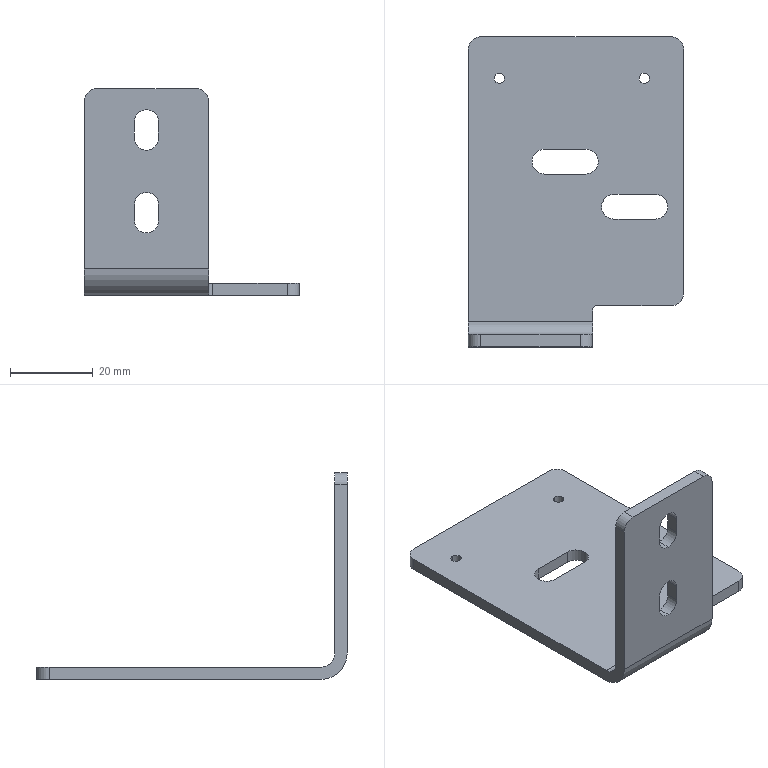Part | STEP file | J014-EBZ05-11-06-Part-1 | 1 solid | 40 faces | box 52 x 75 x 50 mm | volume 14187 mm3 | cylinder 22 | plane 18 | commonest cylinder face diameters 6 x9 5.8 x6 2.5 x4 2 x1 6.4 x1 12.8 x1
STEP:
#1=CARTESIAN_POINT('',(42.5,66.25,0.));
#2=VERTEX_POINT('',#1);
#3=CARTESIAN_POINT('',(42.5,63.75,0.));
#4=VERTEX_POINT('',#3);
#5=CARTESIAN_POINT('',(42.5,65.,0.));
#6=DIRECTION('',(0.,0.,1.));
#7=DIRECTION('',(0.,-1.,0.));
#8=AXIS2_PLACEMENT_3D('',#5,#6,#7);
#9=CIRCLE('',#8,1.25);
#10=EDGE_CURVE('',#2,#4,#9,.T.);
#11=ORIENTED_EDGE('',*,*,#10,.F.);
#12=CARTESIAN_POINT('',(42.5,66.25,3.));
#13=VERTEX_POINT('',#12);
#14=CARTESIAN_POINT('',(42.5,66.25,0.));
#15=DIRECTION('',(0.,0.,1.));
#16=VECTOR('',#15,1000.);
#17=LINE('',#14,#16);
#18=EDGE_CURVE('',#2,#13,#17,.T.);
#19=ORIENTED_EDGE('',*,*,#18,.T.);
#20=CARTESIAN_POINT('',(42.5,63.75,3.));
#21=VERTEX_POINT('',#20);
#22=CARTESIAN_POINT('',(42.5,65.,3.));
#23=DIRECTION('',(0.,0.,-1.));
#24=DIRECTION('',(0.,1.,0.));
#25=AXIS2_PLACEMENT_3D('',#22,#23,#24);
#26=CIRCLE('',#25,1.25);
#27=EDGE_CURVE('',#21,#13,#26,.T.);
#28=ORIENTED_EDGE('',*,*,#27,.F.);
#29=CARTESIAN_POINT('',(42.5,63.75,0.));
#30=DIRECTION('',(0.,0.,1.));
#31=VECTOR('',#30,1000.);
#32=LINE('',#29,#31);
#33=EDGE_CURVE('',#4,#21,#32,.T.);
#34=ORIENTED_EDGE('',*,*,#33,.F.);
#35=EDGE_LOOP('',(#11,#19,#28,#34));
#36=FACE_OUTER_BOUND('',#35,.T.);
#37=CARTESIAN_POINT('',(42.5,65.,0.));
#38=DIRECTION('',(0.,0.,1.));
#39=DIRECTION('',(0.,-1.,0.));
#40=AXIS2_PLACEMENT_3D('',#37,#38,#39);
#41=CYLINDRICAL_SURFACE('',#40,1.25);
#42=ADVANCED_FACE('',(#36),#41,.F.);
#43=CARTESIAN_POINT('',(7.5,66.25,0.));
#44=VERTEX_POINT('',#43);
#45=CARTESIAN_POINT('',(7.5,63.75,0.));
#46=VERTEX_POINT('',#45);
#47=CARTESIAN_POINT('',(7.5,65.,0.));
#48=DIRECTION('',(0.,0.,1.));
#49=DIRECTION('',(0.,-1.,0.));
#50=AXIS2_PLACEMENT_3D('',#47,#48,#49);
#51=CIRCLE('',#50,1.25);
#52=EDGE_CURVE('',#44,#46,#51,.T.);
#53=ORIENTED_EDGE('',*,*,#52,.F.);
#54=CARTESIAN_POINT('',(7.5,66.25,3.));
#55=VERTEX_POINT('',#54);
#56=CARTESIAN_POINT('',(7.5,66.25,0.));
#57=DIRECTION('',(0.,0.,1.));
#58=VECTOR('',#57,1000.);
#59=LINE('',#56,#58);
#60=EDGE_CURVE('',#44,#55,#59,.T.);
#61=ORIENTED_EDGE('',*,*,#60,.T.);
#62=CARTESIAN_POINT('',(7.5,63.75,3.));
#63=VERTEX_POINT('',#62);
#64=CARTESIAN_POINT('',(7.5,65.,3.));
#65=DIRECTION('',(0.,0.,-1.));
#66=DIRECTION('',(0.,1.,0.));
#67=AXIS2_PLACEMENT_3D('',#64,#65,#66);
#68=CIRCLE('',#67,1.25);
#69=EDGE_CURVE('',#63,#55,#68,.T.);
#70=ORIENTED_EDGE('',*,*,#69,.F.);
#71=CARTESIAN_POINT('',(7.5,63.75,0.));
#72=DIRECTION('',(0.,0.,1.));
#73=VECTOR('',#72,1000.);
#74=LINE('',#71,#73);
#75=EDGE_CURVE('',#46,#63,#74,.T.);
#76=ORIENTED_EDGE('',*,*,#75,.F.);
#77=EDGE_LOOP('',(#53,#61,#70,#76));
#78=FACE_OUTER_BOUND('',#77,.T.);
#79=CARTESIAN_POINT('',(7.5,65.,0.));
#80=DIRECTION('',(0.,0.,1.));
#81=DIRECTION('',(0.,-1.,0.));
#82=AXIS2_PLACEMENT_3D('',#79,#80,#81);
#83=CYLINDRICAL_SURFACE('',#82,1.25);
#84=ADVANCED_FACE('',(#78),#83,.F.);
#85=CARTESIAN_POINT('',(15.,3.,35.1));
#86=VERTEX_POINT('',#85);
#87=CARTESIAN_POINT('',(17.9,3.,38.));
#88=VERTEX_POINT('',#87);
#89=CARTESIAN_POINT('',(15.,3.,38.));
#90=DIRECTION('',(0.,-1.,0.));
#91=DIRECTION('',(0.,0.,-1.));
#92=AXIS2_PLACEMENT_3D('',#89,#90,#91);
#93=CIRCLE('',#92,2.9);
#94=EDGE_CURVE('',#86,#88,#93,.T.);
#95=ORIENTED_EDGE('',*,*,#94,.F.);
#96=CARTESIAN_POINT('',(15.,0.,35.1));
#97=VERTEX_POINT('',#96);
#98=CARTESIAN_POINT('',(15.,3.,35.1));
#99=DIRECTION('',(0.,-1.,0.));
#100=VECTOR('',#99,1000.);
#101=LINE('',#98,#100);
#102=EDGE_CURVE('',#86,#97,#101,.T.);
#103=ORIENTED_EDGE('',*,*,#102,.T.);
#104=CARTESIAN_POINT('',(17.9,0.,38.));
#105=VERTEX_POINT('',#104);
#106=CARTESIAN_POINT('',(15.,0.,38.));
#107=DIRECTION('',(0.,1.,0.));
#108=DIRECTION('',(0.,0.,1.));
#109=AXIS2_PLACEMENT_3D('',#106,#107,#108);
#110=CIRCLE('',#109,2.9);
#111=EDGE_CURVE('',#105,#97,#110,.T.);
#112=ORIENTED_EDGE('',*,*,#111,.F.);
#113=CARTESIAN_POINT('',(17.9,3.,38.));
#114=DIRECTION('',(0.,-1.,0.));
#115=VECTOR('',#114,1000.);
#116=LINE('',#113,#115);
#117=EDGE_CURVE('',#88,#105,#116,.T.);
#118=ORIENTED_EDGE('',*,*,#117,.F.);
#119=EDGE_LOOP('',(#95,#103,#112,#118));
#120=FACE_OUTER_BOUND('',#119,.T.);
#121=CARTESIAN_POINT('',(15.,3.,38.));
#122=DIRECTION('',(0.,-1.,0.));
#123=DIRECTION('',(0.,0.,-1.));
#124=AXIS2_PLACEMENT_3D('',#121,#122,#123);
#125=CYLINDRICAL_SURFACE('',#124,2.9);
#126=ADVANCED_FACE('',(#120),#125,.F.);
#127=CARTESIAN_POINT('',(15.,3.,15.1));
#128=VERTEX_POINT('',#127);
#129=CARTESIAN_POINT('',(17.9,3.,18.));
#130=VERTEX_POINT('',#129);
#131=CARTESIAN_POINT('',(15.,3.,18.));
#132=DIRECTION('',(0.,-1.,0.));
#133=DIRECTION('',(0.,0.,-1.));
#134=AXIS2_PLACEMENT_3D('',#131,#132,#133);
#135=CIRCLE('',#134,2.9);
#136=EDGE_CURVE('',#128,#130,#135,.T.);
#137=ORIENTED_EDGE('',*,*,#136,.F.);
#138=CARTESIAN_POINT('',(15.,0.,15.1));
#139=VERTEX_POINT('',#138);
#140=CARTESIAN_POINT('',(15.,3.,15.1));
#141=DIRECTION('',(0.,-1.,0.));
#142=VECTOR('',#141,1000.);
#143=LINE('',#140,#142);
#144=EDGE_CURVE('',#128,#139,#143,.T.);
#145=ORIENTED_EDGE('',*,*,#144,.T.);
#146=CARTESIAN_POINT('',(17.9,0.,18.));
#147=VERTEX_POINT('',#146);
#148=CARTESIAN_POINT('',(15.,0.,18.));
#149=DIRECTION('',(0.,1.,0.));
#150=DIRECTION('',(0.,0.,1.));
#151=AXIS2_PLACEMENT_3D('',#148,#149,#150);
#152=CIRCLE('',#151,2.9);
#153=EDGE_CURVE('',#147,#139,#152,.T.);
#154=ORIENTED_EDGE('',*,*,#153,.F.);
#155=CARTESIAN_POINT('',(17.9,3.,18.));
#156=DIRECTION('',(0.,-1.,0.));
#157=VECTOR('',#156,1000.);
#158=LINE('',#155,#157);
#159=EDGE_CURVE('',#130,#147,#158,.T.);
#160=ORIENTED_EDGE('',*,*,#159,.F.);
#161=EDGE_LOOP('',(#137,#145,#154,#160));
#162=FACE_OUTER_BOUND('',#161,.T.);
#163=CARTESIAN_POINT('',(15.,3.,18.));
#164=DIRECTION('',(0.,-1.,0.));
#165=DIRECTION('',(0.,0.,-1.));
#166=AXIS2_PLACEMENT_3D('',#163,#164,#165);
#167=CYLINDRICAL_SURFACE('',#166,2.9);
#168=ADVANCED_FACE('',(#162),#167,.F.);
#169=CARTESIAN_POINT('',(42.5,65.,0.));
#170=DIRECTION('',(0.,0.,1.));
#171=DIRECTION('',(0.,-1.,0.));
#172=AXIS2_PLACEMENT_3D('',#169,#170,#171);
#173=CIRCLE('',#172,1.25);
#174=EDGE_CURVE('',#4,#2,#173,.T.);
#175=ORIENTED_EDGE('',*,*,#174,.T.);
#176=ORIENTED_EDGE('',*,*,#10,.T.);
#177=EDGE_LOOP('',(#175,#176));
#178=FACE_BOUND('',#177,.T.);
#179=CARTESIAN_POINT('',(7.5,65.,0.));
#180=DIRECTION('',(0.,0.,1.));
#181=DIRECTION('',(0.,-1.,0.));
#182=AXIS2_PLACEMENT_3D('',#179,#180,#181);
#183=CIRCLE('',#182,1.25);
#184=EDGE_CURVE('',#46,#44,#183,.T.);
#185=ORIENTED_EDGE('',*,*,#184,.T.);
#186=ORIENTED_EDGE('',*,*,#52,.T.);
#187=EDGE_LOOP('',(#185,#186));
#188=FACE_BOUND('',#187,.T.);
#189=CARTESIAN_POINT('',(49.,10.,0.));
#190=VERTEX_POINT('',#189);
#191=CARTESIAN_POINT('',(31.,10.,0.));
#192=VERTEX_POINT('',#191);
#193=CARTESIAN_POINT('',(41.,10.,0.));
#194=DIRECTION('',(-1.,0.,0.));
#195=VECTOR('',#194,1000.);
#196=LINE('',#193,#195);
#197=EDGE_CURVE('',#190,#192,#196,.T.);
#198=ORIENTED_EDGE('',*,*,#197,.T.);
#199=CARTESIAN_POINT('',(30.,9.,0.));
#200=VERTEX_POINT('',#199);
#201=CARTESIAN_POINT('',(31.,9.,0.));
#202=DIRECTION('',(0.,0.,1.));
#203=DIRECTION('',(-1.,0.,0.));
#204=AXIS2_PLACEMENT_3D('',#201,#202,#203);
#205=CIRCLE('',#204,1.);
#206=EDGE_CURVE('',#192,#200,#205,.T.);
#207=ORIENTED_EDGE('',*,*,#206,.T.);
#208=CARTESIAN_POINT('',(30.,6.4,0.));
#209=VERTEX_POINT('',#208);
#210=CARTESIAN_POINT('',(30.,5.,0.));
#211=DIRECTION('',(0.,-1.,0.));
#212=VECTOR('',#211,1000.);
#213=LINE('',#210,#212);
#214=EDGE_CURVE('',#200,#209,#213,.T.);
#215=ORIENTED_EDGE('',*,*,#214,.T.);
#216=CARTESIAN_POINT('',(0.,6.4,0.));
#217=VERTEX_POINT('',#216);
#218=CARTESIAN_POINT('',(15.,6.4,0.));
#219=DIRECTION('',(-1.,0.,0.));
#220=VECTOR('',#219,1000.);
#221=LINE('',#218,#220);
#222=EDGE_CURVE('',#209,#217,#221,.T.);
#223=ORIENTED_EDGE('',*,*,#222,.T.);
#224=CARTESIAN_POINT('',(0.,72.,0.));
#225=VERTEX_POINT('',#224);
#226=CARTESIAN_POINT('',(0.,3.,0.));
#227=DIRECTION('',(0.,-1.,0.));
#228=VECTOR('',#227,1000.);
#229=LINE('',#226,#228);
#230=EDGE_CURVE('',#225,#217,#229,.T.);
#231=ORIENTED_EDGE('',*,*,#230,.F.);
#232=CARTESIAN_POINT('',(3.,75.,0.));
#233=VERTEX_POINT('',#232);
#234=CARTESIAN_POINT('',(3.,72.,0.));
#235=DIRECTION('',(0.,0.,-1.));
#236=DIRECTION('',(-1.,0.,0.));
#237=AXIS2_PLACEMENT_3D('',#234,#235,#236);
#238=CIRCLE('',#237,3.);
#239=EDGE_CURVE('',#225,#233,#238,.T.);
#240=ORIENTED_EDGE('',*,*,#239,.T.);
#241=CARTESIAN_POINT('',(49.,75.,0.));
#242=VERTEX_POINT('',#241);
#243=CARTESIAN_POINT('',(26.,75.,0.));
#244=DIRECTION('',(-1.,0.,0.));
#245=VECTOR('',#244,1000.);
#246=LINE('',#243,#245);
#247=EDGE_CURVE('',#242,#233,#246,.T.);
#248=ORIENTED_EDGE('',*,*,#247,.F.);
#249=CARTESIAN_POINT('',(52.,72.,0.));
#250=VERTEX_POINT('',#249);
#251=CARTESIAN_POINT('',(49.,72.,0.));
#252=DIRECTION('',(0.,0.,-1.));
#253=DIRECTION('',(-1.,0.,0.));
#254=AXIS2_PLACEMENT_3D('',#251,#252,#253);
#255=CIRCLE('',#254,3.);
#256=EDGE_CURVE('',#242,#250,#255,.T.);
#257=ORIENTED_EDGE('',*,*,#256,.T.);
#258=CARTESIAN_POINT('',(52.,13.,0.));
#259=VERTEX_POINT('',#258);
#260=CARTESIAN_POINT('',(52.,37.5,0.));
#261=DIRECTION('',(0.,1.,0.));
#262=VECTOR('',#261,1000.);
#263=LINE('',#260,#262);
#264=EDGE_CURVE('',#259,#250,#263,.T.);
#265=ORIENTED_EDGE('',*,*,#264,.F.);
#266=CARTESIAN_POINT('',(49.,13.,0.));
#267=DIRECTION('',(0.,0.,-1.));
#268=DIRECTION('',(-1.,0.,0.));
#269=AXIS2_PLACEMENT_3D('',#266,#267,#268);
#270=CIRCLE('',#269,3.);
#271=EDGE_CURVE('',#259,#190,#270,.T.);
#272=ORIENTED_EDGE('',*,*,#271,.T.);
#273=EDGE_LOOP('',(#198,#207,#215,#223,#231,#240,#248,#257,#265,#272));
#274=FACE_OUTER_BOUND('',#273,.T.);
#275=CARTESIAN_POINT('',(35.169,30.947,0.));
#276=VERTEX_POINT('',#275);
#277=CARTESIAN_POINT('',(45.169,30.947,0.));
#278=VERTEX_POINT('',#277);
#279=CARTESIAN_POINT('',(40.169,30.947,0.));
#280=DIRECTION('',(1.,0.,0.));
#281=VECTOR('',#280,1000.);
#282=LINE('',#279,#281);
#283=EDGE_CURVE('',#276,#278,#282,.T.);
#284=ORIENTED_EDGE('',*,*,#283,.T.);
#285=CARTESIAN_POINT('',(45.169,36.947,0.));
#286=VERTEX_POINT('',#285);
#287=CARTESIAN_POINT('',(45.169,33.947,0.));
#288=DIRECTION('',(0.,0.,1.));
#289=DIRECTION('',(0.,-1.,0.));
#290=AXIS2_PLACEMENT_3D('',#287,#288,#289);
#291=CIRCLE('',#290,3.);
#292=EDGE_CURVE('',#278,#286,#291,.T.);
#293=ORIENTED_EDGE('',*,*,#292,.T.);
#294=CARTESIAN_POINT('',(35.169,36.947,0.));
#295=VERTEX_POINT('',#294);
#296=CARTESIAN_POINT('',(40.169,36.947,0.));
#297=DIRECTION('',(-1.,0.,0.));
#298=VECTOR('',#297,1000.);
#299=LINE('',#296,#298);
#300=EDGE_CURVE('',#286,#295,#299,.T.);
#301=ORIENTED_EDGE('',*,*,#300,.T.);
#302=CARTESIAN_POINT('',(35.169,33.947,0.));
#303=DIRECTION('',(0.,0.,1.));
#304=DIRECTION('',(0.,-1.,0.));
#305=AXIS2_PLACEMENT_3D('',#302,#303,#304);
#306=CIRCLE('',#305,3.);
#307=EDGE_CURVE('',#295,#276,#306,.T.);
#308=ORIENTED_EDGE('',*,*,#307,.T.);
#309=EDGE_LOOP('',(#284,#293,#301,#308));
#310=FACE_BOUND('',#309,.T.);
#311=CARTESIAN_POINT('',(18.396,41.839,0.));
#312=VERTEX_POINT('',#311);
#313=CARTESIAN_POINT('',(28.396,41.839,0.));
#314=VERTEX_POINT('',#313);
#315=CARTESIAN_POINT('',(23.396,41.839,0.));
#316=DIRECTION('',(1.,0.,0.));
#317=VECTOR('',#316,1000.);
#318=LINE('',#315,#317);
#319=EDGE_CURVE('',#312,#314,#318,.T.);
#320=ORIENTED_EDGE('',*,*,#319,.T.);
#321=CARTESIAN_POINT('',(28.396,47.839,0.));
#322=VERTEX_POINT('',#321);
#323=CARTESIAN_POINT('',(28.396,44.839,0.));
#324=DIRECTION('',(0.,0.,1.));
#325=DIRECTION('',(0.,-1.,0.));
#326=AXIS2_PLACEMENT_3D('',#323,#324,#325);
#327=CIRCLE('',#326,3.);
#328=EDGE_CURVE('',#314,#322,#327,.T.);
#329=ORIENTED_EDGE('',*,*,#328,.T.);
#330=CARTESIAN_POINT('',(18.396,47.839,0.));
#331=VERTEX_POINT('',#330);
#332=CARTESIAN_POINT('',(23.396,47.839,0.));
#333=DIRECTION('',(-1.,0.,0.));
#334=VECTOR('',#333,1000.);
#335=LINE('',#332,#334);
#336=EDGE_CURVE('',#322,#331,#335,.T.);
#337=ORIENTED_EDGE('',*,*,#336,.T.);
#338=CARTESIAN_POINT('',(18.396,44.839,0.));
#339=DIRECTION('',(0.,0.,1.));
#340=DIRECTION('',(0.,-1.,0.));
#341=AXIS2_PLACEMENT_3D('',#338,#339,#340);
#342=CIRCLE('',#341,3.);
#343=EDGE_CURVE('',#331,#312,#342,.T.);
#344=ORIENTED_EDGE('',*,*,#343,.T.);
#345=EDGE_LOOP('',(#320,#329,#337,#344));
#346=FACE_BOUND('',#345,.T.);
#347=CARTESIAN_POINT('',(15.,3.,0.));
#348=DIRECTION('',(0.,0.,-1.));
#349=DIRECTION('',(0.,-1.,0.));
#350=AXIS2_PLACEMENT_3D('',#347,#348,#349);
#351=PLANE('',#350);
#352=ADVANCED_FACE('',(#178,#188,#274,#310,#346),#351,.T.);
#353=CARTESIAN_POINT('',(28.396,41.839,3.));
#354=VERTEX_POINT('',#353);
#355=CARTESIAN_POINT('',(28.396,47.839,3.));
#356=VERTEX_POINT('',#355);
#357=CARTESIAN_POINT('',(28.396,44.839,3.));
#358=DIRECTION('',(0.,0.,1.));
#359=DIRECTION('',(0.,-1.,0.));
#360=AXIS2_PLACEMENT_3D('',#357,#358,#359);
#361=CIRCLE('',#360,3.);
#362=EDGE_CURVE('',#354,#356,#361,.T.);
#363=ORIENTED_EDGE('',*,*,#362,.F.);
#364=CARTESIAN_POINT('',(18.396,41.839,3.));
#365=VERTEX_POINT('',#364);
#366=CARTESIAN_POINT('',(26.,41.839,3.));
#367=DIRECTION('',(1.,0.,0.));
#368=VECTOR('',#367,1000.);
#369=LINE('',#366,#368);
#370=EDGE_CURVE('',#365,#354,#369,.T.);
#371=ORIENTED_EDGE('',*,*,#370,.F.);
#372=CARTESIAN_POINT('',(18.396,47.839,3.));
#373=VERTEX_POINT('',#372);
#374=CARTESIAN_POINT('',(18.396,44.839,3.));
#375=DIRECTION('',(0.,0.,1.));
#376=DIRECTION('',(0.,-1.,0.));
#377=AXIS2_PLACEMENT_3D('',#374,#375,#376);
#378=CIRCLE('',#377,3.);
#379=EDGE_CURVE('',#373,#365,#378,.T.);
#380=ORIENTED_EDGE('',*,*,#379,.F.);
#381=CARTESIAN_POINT('',(26.,47.839,3.));
#382=DIRECTION('',(-1.,0.,0.));
#383=VECTOR('',#382,1000.);
#384=LINE('',#381,#383);
#385=EDGE_CURVE('',#356,#373,#384,.T.);
#386=ORIENTED_EDGE('',*,*,#385,.F.);
#387=EDGE_LOOP('',(#363,#371,#380,#386));
#388=FACE_BOUND('',#387,.T.);
#389=CARTESIAN_POINT('',(45.169,30.947,3.));
#390=VERTEX_POINT('',#389);
#391=CARTESIAN_POINT('',(45.169,36.947,3.));
#392=VERTEX_POINT('',#391);
#393=CARTESIAN_POINT('',(45.169,33.947,3.));
#394=DIRECTION('',(0.,0.,1.));
#395=DIRECTION('',(0.,-1.,0.));
#396=AXIS2_PLACEMENT_3D('',#393,#394,#395);
#397=CIRCLE('',#396,3.);
#398=EDGE_CURVE('',#390,#392,#397,.T.);
#399=ORIENTED_EDGE('',*,*,#398,.F.);
#400=CARTESIAN_POINT('',(35.169,30.947,3.));
#401=VERTEX_POINT('',#400);
#402=CARTESIAN_POINT('',(26.,30.947,3.));
#403=DIRECTION('',(1.,0.,0.));
#404=VECTOR('',#403,1000.);
#405=LINE('',#402,#404);
#406=EDGE_CURVE('',#401,#390,#405,.T.);
#407=ORIENTED_EDGE('',*,*,#406,.F.);
#408=CARTESIAN_POINT('',(35.169,36.947,3.));
#409=VERTEX_POINT('',#408);
#410=CARTESIAN_POINT('',(35.169,33.947,3.));
#411=DIRECTION('',(0.,0.,1.));
#412=DIRECTION('',(0.,-1.,0.));
#413=AXIS2_PLACEMENT_3D('',#410,#411,#412);
#414=CIRCLE('',#413,3.);
#415=EDGE_CURVE('',#409,#401,#414,.T.);
#416=ORIENTED_EDGE('',*,*,#415,.F.);
#417=CARTESIAN_POINT('',(26.,36.947,3.));
#418=DIRECTION('',(-1.,0.,0.));
#419=VECTOR('',#418,1000.);
#420=LINE('',#417,#419);
#421=EDGE_CURVE('',#392,#409,#420,.T.);
#422=ORIENTED_EDGE('',*,*,#421,.F.);
#423=EDGE_LOOP('',(#399,#407,#416,#422));
#424=FACE_BOUND('',#423,.T.);
#425=ORIENTED_EDGE('',*,*,#27,.T.);
#426=CARTESIAN_POINT('',(42.5,65.,3.));
#427=DIRECTION('',(0.,0.,-1.));
#428=DIRECTION('',(0.,1.,0.));
#429=AXIS2_PLACEMENT_3D('',#426,#427,#428);
#430=CIRCLE('',#429,1.25);
#431=EDGE_CURVE('',#13,#21,#430,.T.);
#432=ORIENTED_EDGE('',*,*,#431,.T.);
#433=EDGE_LOOP('',(#425,#432));
#434=FACE_BOUND('',#433,.T.);
#435=ORIENTED_EDGE('',*,*,#69,.T.);
#436=CARTESIAN_POINT('',(7.5,65.,3.));
#437=DIRECTION('',(0.,0.,-1.));
#438=DIRECTION('',(0.,1.,0.));
#439=AXIS2_PLACEMENT_3D('',#436,#437,#438);
#440=CIRCLE('',#439,1.25);
#441=EDGE_CURVE('',#55,#63,#440,.T.);
#442=ORIENTED_EDGE('',*,*,#441,.T.);
#443=EDGE_LOOP('',(#435,#442));
#444=FACE_BOUND('',#443,.T.);
#445=CARTESIAN_POINT('',(0.,6.2,3.));
#446=VERTEX_POINT('',#445);
#447=CARTESIAN_POINT('',(0.,72.,3.));
#448=VERTEX_POINT('',#447);
#449=CARTESIAN_POINT('',(0.,37.5,3.));
#450=DIRECTION('',(0.,1.,0.));
#451=VECTOR('',#450,1000.);
#452=LINE('',#449,#451);
#453=EDGE_CURVE('',#446,#448,#452,.T.);
#454=ORIENTED_EDGE('',*,*,#453,.F.);
#455=CARTESIAN_POINT('',(30.,6.2,3.));
#456=VERTEX_POINT('',#455);
#457=CARTESIAN_POINT('',(30.,6.2,3.));
#458=DIRECTION('',(1.,0.,0.));
#459=VECTOR('',#458,1000.);
#460=LINE('',#457,#459);
#461=EDGE_CURVE('',#446,#456,#460,.T.);
#462=ORIENTED_EDGE('',*,*,#461,.T.);
#463=CARTESIAN_POINT('',(30.,9.,3.));
#464=VERTEX_POINT('',#463);
#465=CARTESIAN_POINT('',(30.,5.,3.));
#466=DIRECTION('',(0.,1.,0.));
#467=VECTOR('',#466,1000.);
#468=LINE('',#465,#467);
#469=EDGE_CURVE('',#456,#464,#468,.T.);
#470=ORIENTED_EDGE('',*,*,#469,.T.);
#471=CARTESIAN_POINT('',(31.,10.,3.));
#472=VERTEX_POINT('',#471);
#473=CARTESIAN_POINT('',(31.,9.,3.));
#474=DIRECTION('',(0.,0.,-1.));
#475=DIRECTION('',(0.,-1.,0.));
#476=AXIS2_PLACEMENT_3D('',#473,#474,#475);
#477=CIRCLE('',#476,1.);
#478=EDGE_CURVE('',#464,#472,#477,.T.);
#479=ORIENTED_EDGE('',*,*,#478,.T.);
#480=CARTESIAN_POINT('',(49.,10.,3.));
#481=VERTEX_POINT('',#480);
#482=CARTESIAN_POINT('',(41.,10.,3.));
#483=DIRECTION('',(1.,0.,0.));
#484=VECTOR('',#483,1000.);
#485=LINE('',#482,#484);
#486=EDGE_CURVE('',#472,#481,#485,.T.);
#487=ORIENTED_EDGE('',*,*,#486,.T.);
#488=CARTESIAN_POINT('',(52.,13.,3.));
#489=VERTEX_POINT('',#488);
#490=CARTESIAN_POINT('',(49.,13.,3.));
#491=DIRECTION('',(0.,0.,1.));
#492=DIRECTION('',(0.,-1.,0.));
#493=AXIS2_PLACEMENT_3D('',#490,#491,#492);
#494=CIRCLE('',#493,3.);
#495=EDGE_CURVE('',#481,#489,#494,.T.);
#496=ORIENTED_EDGE('',*,*,#495,.T.);
#497=CARTESIAN_POINT('',(52.,72.,3.));
#498=VERTEX_POINT('',#497);
#499=CARTESIAN_POINT('',(52.,37.5,3.));
#500=DIRECTION('',(0.,-1.,0.));
#501=VECTOR('',#500,1000.);
#502=LINE('',#499,#501);
#503=EDGE_CURVE('',#498,#489,#502,.T.);
#504=ORIENTED_EDGE('',*,*,#503,.F.);
#505=CARTESIAN_POINT('',(49.,75.,3.));
#506=VERTEX_POINT('',#505);
#507=CARTESIAN_POINT('',(49.,72.,3.));
#508=DIRECTION('',(0.,0.,1.));
#509=DIRECTION('',(0.,-1.,0.));
#510=AXIS2_PLACEMENT_3D('',#507,#508,#509);
#511=CIRCLE('',#510,3.);
#512=EDGE_CURVE('',#498,#506,#511,.T.);
#513=ORIENTED_EDGE('',*,*,#512,.T.);
#514=CARTESIAN_POINT('',(3.,75.,3.));
#515=VERTEX_POINT('',#514);
#516=CARTESIAN_POINT('',(26.,75.,3.));
#517=DIRECTION('',(1.,0.,0.));
#518=VECTOR('',#517,1000.);
#519=LINE('',#516,#518);
#520=EDGE_CURVE('',#515,#506,#519,.T.);
#521=ORIENTED_EDGE('',*,*,#520,.F.);
#522=CARTESIAN_POINT('',(3.,72.,3.));
#523=DIRECTION('',(0.,0.,1.));
#524=DIRECTION('',(0.,-1.,0.));
#525=AXIS2_PLACEMENT_3D('',#522,#523,#524);
#526=CIRCLE('',#525,3.);
#527=EDGE_CURVE('',#515,#448,#526,.T.);
#528=ORIENTED_EDGE('',*,*,#527,.T.);
#529=EDGE_LOOP('',(#454,#462,#470,#479,#487,#496,#504,#513,#521,#528));
#530=FACE_OUTER_BOUND('',#529,.T.);
#531=CARTESIAN_POINT('',(26.,37.5,3.));
#532=DIRECTION('',(0.,0.,1.));
#533=DIRECTION('',(-1.,0.,0.));
#534=AXIS2_PLACEMENT_3D('',#531,#532,#533);
#535=PLANE('',#534);
#536=ADVANCED_FACE('',(#388,#424,#434,#444,#530),#535,.T.);
#537=ORIENTED_EDGE('',*,*,#503,.T.);
#538=CARTESIAN_POINT('',(52.,13.,0.));
#539=DIRECTION('',(0.,0.,-1.));
#540=VECTOR('',#539,1000.);
#541=LINE('',#538,#540);
#542=EDGE_CURVE('',#489,#259,#541,.T.);
#543=ORIENTED_EDGE('',*,*,#542,.T.);
#544=ORIENTED_EDGE('',*,*,#264,.T.);
#545=CARTESIAN_POINT('',(52.,72.,0.));
#546=DIRECTION('',(0.,0.,1.));
#547=VECTOR('',#546,1000.);
#548=LINE('',#545,#547);
#549=EDGE_CURVE('',#250,#498,#548,.T.);
#550=ORIENTED_EDGE('',*,*,#549,.T.);
#551=EDGE_LOOP('',(#537,#543,#544,#550));
#552=FACE_OUTER_BOUND('',#551,.T.);
#553=CARTESIAN_POINT('',(52.,37.5,0.));
#554=DIRECTION('',(1.,0.,0.));
#555=DIRECTION('',(0.,0.,1.));
#556=AXIS2_PLACEMENT_3D('',#553,#554,#555);
#557=PLANE('',#556);
#558=ADVANCED_FACE('',(#552),#557,.T.);
#559=CARTESIAN_POINT('',(0.,0.,6.4));
#560=VERTEX_POINT('',#559);
#561=CARTESIAN_POINT('',(0.,0.,47.));
#562=VERTEX_POINT('',#561);
#563=CARTESIAN_POINT('',(0.,0.,25.));
#564=DIRECTION('',(0.,0.,1.));
#565=VECTOR('',#564,1000.);
#566=LINE('',#563,#565);
#567=EDGE_CURVE('',#560,#562,#566,.T.);
#568=ORIENTED_EDGE('',*,*,#567,.F.);
#569=CARTESIAN_POINT('',(30.,0.,6.4));
#570=VERTEX_POINT('',#569);
#571=CARTESIAN_POINT('',(15.,0.,6.4));
#572=DIRECTION('',(1.,0.,0.));
#573=VECTOR('',#572,1000.);
#574=LINE('',#571,#573);
#575=EDGE_CURVE('',#560,#570,#574,.T.);
#576=ORIENTED_EDGE('',*,*,#575,.T.);
#577=CARTESIAN_POINT('',(30.,0.,47.));
#578=VERTEX_POINT('',#577);
#579=CARTESIAN_POINT('',(30.,0.,25.));
#580=DIRECTION('',(0.,0.,-1.));
#581=VECTOR('',#580,1000.);
#582=LINE('',#579,#581);
#583=EDGE_CURVE('',#578,#570,#582,.T.);
#584=ORIENTED_EDGE('',*,*,#583,.F.);
#585=CARTESIAN_POINT('',(27.,0.,50.));
#586=VERTEX_POINT('',#585);
#587=CARTESIAN_POINT('',(27.,0.,47.));
#588=DIRECTION('',(0.,-1.,0.));
#589=DIRECTION('',(-1.,0.,0.));
#590=AXIS2_PLACEMENT_3D('',#587,#588,#589);
#591=CIRCLE('',#590,3.);
#592=EDGE_CURVE('',#578,#586,#591,.T.);
#593=ORIENTED_EDGE('',*,*,#592,.T.);
#594=CARTESIAN_POINT('',(3.,0.,50.));
#595=VERTEX_POINT('',#594);
#596=CARTESIAN_POINT('',(15.,0.,50.));
#597=DIRECTION('',(1.,0.,0.));
#598=VECTOR('',#597,1000.);
#599=LINE('',#596,#598);
#600=EDGE_CURVE('',#595,#586,#599,.T.);
#601=ORIENTED_EDGE('',*,*,#600,.F.);
#602=CARTESIAN_POINT('',(3.,0.,47.));
#603=DIRECTION('',(0.,-1.,0.));
#604=DIRECTION('',(-1.,0.,0.));
#605=AXIS2_PLACEMENT_3D('',#602,#603,#604);
#606=CIRCLE('',#605,3.);
#607=EDGE_CURVE('',#595,#562,#606,.T.);
#608=ORIENTED_EDGE('',*,*,#607,.T.);
#609=EDGE_LOOP('',(#568,#576,#584,#593,#601,#608));
#610=FACE_OUTER_BOUND('',#609,.T.);
#611=CARTESIAN_POINT('',(12.1,0.,18.));
#612=VERTEX_POINT('',#611);
#613=CARTESIAN_POINT('',(12.1,0.,22.));
#614=VERTEX_POINT('',#613);
#615=CARTESIAN_POINT('',(12.1,0.,20.));
#616=DIRECTION('',(0.,0.,1.));
#617=VECTOR('',#616,1000.);
#618=LINE('',#615,#617);
#619=EDGE_CURVE('',#612,#614,#618,.T.);
#620=ORIENTED_EDGE('',*,*,#619,.T.);
#621=CARTESIAN_POINT('',(17.9,0.,22.));
#622=VERTEX_POINT('',#621);
#623=CARTESIAN_POINT('',(15.,0.,22.));
#624=DIRECTION('',(0.,1.,0.));
#625=DIRECTION('',(0.,0.,1.));
#626=AXIS2_PLACEMENT_3D('',#623,#624,#625);
#627=CIRCLE('',#626,2.9);
#628=EDGE_CURVE('',#614,#622,#627,.T.);
#629=ORIENTED_EDGE('',*,*,#628,.T.);
#630=CARTESIAN_POINT('',(17.9,0.,20.));
#631=DIRECTION('',(0.,0.,-1.));
#632=VECTOR('',#631,1000.);
#633=LINE('',#630,#632);
#634=EDGE_CURVE('',#622,#147,#633,.T.);
#635=ORIENTED_EDGE('',*,*,#634,.T.);
#636=ORIENTED_EDGE('',*,*,#153,.T.);
#637=CARTESIAN_POINT('',(15.,0.,18.));
#638=DIRECTION('',(0.,1.,0.));
#639=DIRECTION('',(0.,0.,1.));
#640=AXIS2_PLACEMENT_3D('',#637,#638,#639);
#641=CIRCLE('',#640,2.9);
#642=EDGE_CURVE('',#139,#612,#641,.T.);
#643=ORIENTED_EDGE('',*,*,#642,.T.);
#644=EDGE_LOOP('',(#620,#629,#635,#636,#643));
#645=FACE_BOUND('',#644,.T.);
#646=CARTESIAN_POINT('',(12.1,0.,38.));
#647=VERTEX_POINT('',#646);
#648=CARTESIAN_POINT('',(12.1,0.,42.));
#649=VERTEX_POINT('',#648);
#650=CARTESIAN_POINT('',(12.1,0.,40.));
#651=DIRECTION('',(0.,0.,1.));
#652=VECTOR('',#651,1000.);
#653=LINE('',#650,#652);
#654=EDGE_CURVE('',#647,#649,#653,.T.);
#655=ORIENTED_EDGE('',*,*,#654,.T.);
#656=CARTESIAN_POINT('',(17.9,0.,42.));
#657=VERTEX_POINT('',#656);
#658=CARTESIAN_POINT('',(15.,0.,42.));
#659=DIRECTION('',(0.,1.,0.));
#660=DIRECTION('',(0.,0.,1.));
#661=AXIS2_PLACEMENT_3D('',#658,#659,#660);
#662=CIRCLE('',#661,2.9);
#663=EDGE_CURVE('',#649,#657,#662,.T.);
#664=ORIENTED_EDGE('',*,*,#663,.T.);
#665=CARTESIAN_POINT('',(17.9,0.,40.));
#666=DIRECTION('',(0.,0.,-1.));
#667=VECTOR('',#666,1000.);
#668=LINE('',#665,#667);
#669=EDGE_CURVE('',#657,#105,#668,.T.);
#670=ORIENTED_EDGE('',*,*,#669,.T.);
#671=ORIENTED_EDGE('',*,*,#111,.T.);
#672=CARTESIAN_POINT('',(15.,0.,38.));
#673=DIRECTION('',(0.,1.,0.));
#674=DIRECTION('',(0.,0.,1.));
#675=AXIS2_PLACEMENT_3D('',#672,#673,#674);
#676=CIRCLE('',#675,2.9);
#677=EDGE_CURVE('',#97,#647,#676,.T.);
#678=ORIENTED_EDGE('',*,*,#677,.T.);
#679=EDGE_LOOP('',(#655,#664,#670,#671,#678));
#680=FACE_BOUND('',#679,.T.);
#681=CARTESIAN_POINT('',(15.,0.,25.));
#682=DIRECTION('',(0.,-1.,0.));
#683=DIRECTION('',(-1.,0.,0.));
#684=AXIS2_PLACEMENT_3D('',#681,#682,#683);
#685=PLANE('',#684);
#686=ADVANCED_FACE('',(#610,#645,#680),#685,.T.);
#687=CARTESIAN_POINT('',(30.,3.,6.2));
#688=VERTEX_POINT('',#687);
#689=CARTESIAN_POINT('',(30.,3.,47.));
#690=VERTEX_POINT('',#689);
#691=CARTESIAN_POINT('',(30.,3.,25.));
#692=DIRECTION('',(0.,0.,1.));
#693=VECTOR('',#692,1000.);
#694=LINE('',#691,#693);
#695=EDGE_CURVE('',#688,#690,#694,.T.);
#696=ORIENTED_EDGE('',*,*,#695,.F.);
#697=CARTESIAN_POINT('',(0.,3.,6.2));
#698=VERTEX_POINT('',#697);
#699=CARTESIAN_POINT('',(0.,3.,6.2));
#700=DIRECTION('',(-1.,0.,0.));
#701=VECTOR('',#700,1000.);
#702=LINE('',#699,#701);
#703=EDGE_CURVE('',#688,#698,#702,.T.);
#704=ORIENTED_EDGE('',*,*,#703,.T.);
#705=CARTESIAN_POINT('',(0.,3.,47.));
#706=VERTEX_POINT('',#705);
#707=CARTESIAN_POINT('',(0.,3.,25.));
#708=DIRECTION('',(0.,0.,-1.));
#709=VECTOR('',#708,1000.);
#710=LINE('',#707,#709);
#711=EDGE_CURVE('',#706,#698,#710,.T.);
#712=ORIENTED_EDGE('',*,*,#711,.F.);
#713=CARTESIAN_POINT('',(3.,3.,50.));
#714=VERTEX_POINT('',#713);
#715=CARTESIAN_POINT('',(3.,3.,47.));
#716=DIRECTION('',(0.,1.,0.));
#717=DIRECTION('',(1.,0.,0.));
#718=AXIS2_PLACEMENT_3D('',#715,#716,#717);
#719=CIRCLE('',#718,3.);
#720=EDGE_CURVE('',#706,#714,#719,.T.);
#721=ORIENTED_EDGE('',*,*,#720,.T.);
#722=CARTESIAN_POINT('',(27.,3.,50.));
#723=VERTEX_POINT('',#722);
#724=CARTESIAN_POINT('',(15.,3.,50.));
#725=DIRECTION('',(-1.,0.,0.));
#726=VECTOR('',#725,1000.);
#727=LINE('',#724,#726);
#728=EDGE_CURVE('',#723,#714,#727,.T.);
#729=ORIENTED_EDGE('',*,*,#728,.F.);
#730=CARTESIAN_POINT('',(27.,3.,47.));
#731=DIRECTION('',(0.,1.,0.));
#732=DIRECTION('',(1.,0.,0.));
#733=AXIS2_PLACEMENT_3D('',#730,#731,#732);
#734=CIRCLE('',#733,3.);
#735=EDGE_CURVE('',#723,#690,#734,.T.);
#736=ORIENTED_EDGE('',*,*,#735,.T.);
#737=EDGE_LOOP('',(#696,#704,#712,#721,#729,#736));
#738=FACE_OUTER_BOUND('',#737,.T.);
#739=CARTESIAN_POINT('',(17.9,3.,22.));
#740=VERTEX_POINT('',#739);
#741=CARTESIAN_POINT('',(17.9,3.,20.));
#742=DIRECTION('',(0.,0.,1.));
#743=VECTOR('',#742,1000.);
#744=LINE('',#741,#743);
#745=EDGE_CURVE('',#130,#740,#744,.T.);
#746=ORIENTED_EDGE('',*,*,#745,.T.);
#747=CARTESIAN_POINT('',(12.1,3.,22.));
#748=VERTEX_POINT('',#747);
#749=CARTESIAN_POINT('',(15.,3.,22.));
#750=DIRECTION('',(0.,-1.,0.));
#751=DIRECTION('',(0.,0.,-1.));
#752=AXIS2_PLACEMENT_3D('',#749,#750,#751);
#753=CIRCLE('',#752,2.9);
#754=EDGE_CURVE('',#740,#748,#753,.T.);
#755=ORIENTED_EDGE('',*,*,#754,.T.);
#756=CARTESIAN_POINT('',(12.1,3.,18.));
#757=VERTEX_POINT('',#756);
#758=CARTESIAN_POINT('',(12.1,3.,20.));
#759=DIRECTION('',(0.,0.,-1.));
#760=VECTOR('',#759,1000.);
#761=LINE('',#758,#760);
#762=EDGE_CURVE('',#748,#757,#761,.T.);
#763=ORIENTED_EDGE('',*,*,#762,.T.);
#764=CARTESIAN_POINT('',(15.,3.,18.));
#765=DIRECTION('',(0.,-1.,0.));
#766=DIRECTION('',(0.,0.,-1.));
#767=AXIS2_PLACEMENT_3D('',#764,#765,#766);
#768=CIRCLE('',#767,2.9);
#769=EDGE_CURVE('',#757,#128,#768,.T.);
#770=ORIENTED_EDGE('',*,*,#769,.T.);
#771=ORIENTED_EDGE('',*,*,#136,.T.);
#772=EDGE_LOOP('',(#746,#755,#763,#770,#771));
#773=FACE_BOUND('',#772,.T.);
#774=CARTESIAN_POINT('',(17.9,3.,42.));
#775=VERTEX_POINT('',#774);
#776=CARTESIAN_POINT('',(17.9,3.,40.));
#777=DIRECTION('',(0.,0.,1.));
#778=VECTOR('',#777,1000.);
#779=LINE('',#776,#778);
#780=EDGE_CURVE('',#88,#775,#779,.T.);
#781=ORIENTED_EDGE('',*,*,#780,.T.);
#782=CARTESIAN_POINT('',(12.1,3.,42.));
#783=VERTEX_POINT('',#782);
#784=CARTESIAN_POINT('',(15.,3.,42.));
#785=DIRECTION('',(0.,-1.,0.));
#786=DIRECTION('',(0.,0.,-1.));
#787=AXIS2_PLACEMENT_3D('',#784,#785,#786);
#788=CIRCLE('',#787,2.9);
#789=EDGE_CURVE('',#775,#783,#788,.T.);
#790=ORIENTED_EDGE('',*,*,#789,.T.);
#791=CARTESIAN_POINT('',(12.1,3.,38.));
#792=VERTEX_POINT('',#791);
#793=CARTESIAN_POINT('',(12.1,3.,40.));
#794=DIRECTION('',(0.,0.,-1.));
#795=VECTOR('',#794,1000.);
#796=LINE('',#793,#795);
#797=EDGE_CURVE('',#783,#792,#796,.T.);
#798=ORIENTED_EDGE('',*,*,#797,.T.);
#799=CARTESIAN_POINT('',(15.,3.,38.));
#800=DIRECTION('',(0.,-1.,0.));
#801=DIRECTION('',(0.,0.,-1.));
#802=AXIS2_PLACEMENT_3D('',#799,#800,#801);
#803=CIRCLE('',#802,2.9);
#804=EDGE_CURVE('',#792,#86,#803,.T.);
#805=ORIENTED_EDGE('',*,*,#804,.T.);
#806=ORIENTED_EDGE('',*,*,#94,.T.);
#807=EDGE_LOOP('',(#781,#790,#798,#805,#806));
#808=FACE_BOUND('',#807,.T.);
#809=CARTESIAN_POINT('',(15.,3.,25.));
#810=DIRECTION('',(0.,1.,0.));
#811=DIRECTION('',(1.,0.,0.));
#812=AXIS2_PLACEMENT_3D('',#809,#810,#811);
#813=PLANE('',#812);
#814=ADVANCED_FACE('',(#738,#773,#808),#813,.T.);
#815=ORIENTED_EDGE('',*,*,#728,.T.);
#816=CARTESIAN_POINT('',(3.,3.,50.));
#817=DIRECTION('',(0.,-1.,0.));
#818=VECTOR('',#817,1000.);
#819=LINE('',#816,#818);
#820=EDGE_CURVE('',#714,#595,#819,.T.);
#821=ORIENTED_EDGE('',*,*,#820,.T.);
#822=ORIENTED_EDGE('',*,*,#600,.T.);
#823=CARTESIAN_POINT('',(27.,3.,50.));
#824=DIRECTION('',(0.,1.,0.));
#825=VECTOR('',#824,1000.);
#826=LINE('',#823,#825);
#827=EDGE_CURVE('',#586,#723,#826,.T.);
#828=ORIENTED_EDGE('',*,*,#827,.T.);
#829=EDGE_LOOP('',(#815,#821,#822,#828));
#830=FACE_OUTER_BOUND('',#829,.T.);
#831=CARTESIAN_POINT('',(15.,3.,50.));
#832=DIRECTION('',(0.,0.,1.));
#833=DIRECTION('',(0.,1.,0.));
#834=AXIS2_PLACEMENT_3D('',#831,#832,#833);
#835=PLANE('',#834);
#836=ADVANCED_FACE('',(#830),#835,.T.);
#837=ORIENTED_EDGE('',*,*,#214,.F.);
#838=CARTESIAN_POINT('',(30.,9.,25.));
#839=DIRECTION('',(0.,0.,1.));
#840=VECTOR('',#839,1000.);
#841=LINE('',#838,#840);
#842=EDGE_CURVE('',#200,#464,#841,.T.);
#843=ORIENTED_EDGE('',*,*,#842,.T.);
#844=ORIENTED_EDGE('',*,*,#469,.F.);
#845=CARTESIAN_POINT('',(30.,6.2,6.2));
#846=DIRECTION('',(-1.,0.,0.));
#847=DIRECTION('',(0.,0.,-1.));
#848=AXIS2_PLACEMENT_3D('',#845,#846,#847);
#849=CIRCLE('',#848,3.2);
#850=EDGE_CURVE('',#456,#688,#849,.T.);
#851=ORIENTED_EDGE('',*,*,#850,.T.);
#852=ORIENTED_EDGE('',*,*,#695,.T.);
#853=CARTESIAN_POINT('',(30.,3.,47.));
#854=DIRECTION('',(0.,-1.,0.));
#855=VECTOR('',#854,1000.);
#856=LINE('',#853,#855);
#857=EDGE_CURVE('',#690,#578,#856,.T.);
#858=ORIENTED_EDGE('',*,*,#857,.T.);
#859=ORIENTED_EDGE('',*,*,#583,.T.);
#860=CARTESIAN_POINT('',(30.,6.4,6.4));
#861=DIRECTION('',(1.,0.,0.));
#862=DIRECTION('',(0.,0.,-1.));
#863=AXIS2_PLACEMENT_3D('',#860,#861,#862);
#864=CIRCLE('',#863,6.4);
#865=EDGE_CURVE('',#570,#209,#864,.T.);
#866=ORIENTED_EDGE('',*,*,#865,.T.);
#867=EDGE_LOOP('',(#837,#843,#844,#851,#852,#858,#859,#866));
#868=FACE_OUTER_BOUND('',#867,.T.);
#869=CARTESIAN_POINT('',(30.,3.,25.));
#870=DIRECTION('',(1.,0.,0.));
#871=DIRECTION('',(0.,-1.,0.));
#872=AXIS2_PLACEMENT_3D('',#869,#870,#871);
#873=PLANE('',#872);
#874=ADVANCED_FACE('',(#868),#873,.T.);
#875=ORIENTED_EDGE('',*,*,#230,.T.);
#876=CARTESIAN_POINT('',(0.,6.4,6.4));
#877=DIRECTION('',(-1.,0.,0.));
#878=DIRECTION('',(0.,0.,1.));
#879=AXIS2_PLACEMENT_3D('',#876,#877,#878);
#880=CIRCLE('',#879,6.4);
#881=EDGE_CURVE('',#217,#560,#880,.T.);
#882=ORIENTED_EDGE('',*,*,#881,.T.);
#883=ORIENTED_EDGE('',*,*,#567,.T.);
#884=CARTESIAN_POINT('',(0.,3.,47.));
#885=DIRECTION('',(0.,1.,0.));
#886=VECTOR('',#885,1000.);
#887=LINE('',#884,#886);
#888=EDGE_CURVE('',#562,#706,#887,.T.);
#889=ORIENTED_EDGE('',*,*,#888,.T.);
#890=ORIENTED_EDGE('',*,*,#711,.T.);
#891=CARTESIAN_POINT('',(0.,6.2,6.2));
#892=DIRECTION('',(1.,0.,0.));
#893=DIRECTION('',(0.,0.,1.));
#894=AXIS2_PLACEMENT_3D('',#891,#892,#893);
#895=CIRCLE('',#894,3.2);
#896=EDGE_CURVE('',#698,#446,#895,.T.);
#897=ORIENTED_EDGE('',*,*,#896,.T.);
#898=ORIENTED_EDGE('',*,*,#453,.T.);
#899=CARTESIAN_POINT('',(0.,72.,25.));
#900=DIRECTION('',(0.,0.,-1.));
#901=VECTOR('',#900,1000.);
#902=LINE('',#899,#901);
#903=EDGE_CURVE('',#448,#225,#902,.T.);
#904=ORIENTED_EDGE('',*,*,#903,.T.);
#905=EDGE_LOOP('',(#875,#882,#883,#889,#890,#897,#898,#904));
#906=FACE_OUTER_BOUND('',#905,.T.);
#907=CARTESIAN_POINT('',(0.,3.,25.));
#908=DIRECTION('',(-1.,0.,0.));
#909=DIRECTION('',(0.,1.,0.));
#910=AXIS2_PLACEMENT_3D('',#907,#908,#909);
#911=PLANE('',#910);
#912=ADVANCED_FACE('',(#906),#911,.T.);
#913=ORIENTED_EDGE('',*,*,#520,.T.);
#914=CARTESIAN_POINT('',(49.,75.,0.));
#915=DIRECTION('',(0.,0.,-1.));
#916=VECTOR('',#915,1000.);
#917=LINE('',#914,#916);
#918=EDGE_CURVE('',#506,#242,#917,.T.);
#919=ORIENTED_EDGE('',*,*,#918,.T.);
#920=ORIENTED_EDGE('',*,*,#247,.T.);
#921=CARTESIAN_POINT('',(3.,75.,0.));
#922=DIRECTION('',(0.,0.,1.));
#923=VECTOR('',#922,1000.);
#924=LINE('',#921,#923);
#925=EDGE_CURVE('',#233,#515,#924,.T.);
#926=ORIENTED_EDGE('',*,*,#925,.T.);
#927=EDGE_LOOP('',(#913,#919,#920,#926));
#928=FACE_OUTER_BOUND('',#927,.T.);
#929=CARTESIAN_POINT('',(26.,75.,0.));
#930=DIRECTION('',(0.,1.,0.));
#931=DIRECTION('',(0.,0.,-1.));
#932=AXIS2_PLACEMENT_3D('',#929,#930,#931);
#933=PLANE('',#932);
#934=ADVANCED_FACE('',(#928),#933,.T.);
#935=CARTESIAN_POINT('',(17.9,3.,22.));
#936=DIRECTION('',(0.,-1.,0.));
#937=VECTOR('',#936,1000.);
#938=LINE('',#935,#937);
#939=EDGE_CURVE('',#740,#622,#938,.T.);
#940=ORIENTED_EDGE('',*,*,#939,.F.);
#941=ORIENTED_EDGE('',*,*,#745,.F.);
#942=ORIENTED_EDGE('',*,*,#159,.T.);
#943=ORIENTED_EDGE('',*,*,#634,.F.);
#944=EDGE_LOOP('',(#940,#941,#942,#943));
#945=FACE_OUTER_BOUND('',#944,.T.);
#946=CARTESIAN_POINT('',(17.9,3.,20.));
#947=DIRECTION('',(1.,0.,0.));
#948=DIRECTION('',(0.,1.,0.));
#949=AXIS2_PLACEMENT_3D('',#946,#947,#948);
#950=PLANE('',#949);
#951=ADVANCED_FACE('',(#945),#950,.F.);
#952=CARTESIAN_POINT('',(12.1,3.,18.));
#953=DIRECTION('',(0.,-1.,0.));
#954=VECTOR('',#953,1000.);
#955=LINE('',#952,#954);
#956=EDGE_CURVE('',#757,#612,#955,.T.);
#957=ORIENTED_EDGE('',*,*,#956,.F.);
#958=ORIENTED_EDGE('',*,*,#762,.F.);
#959=CARTESIAN_POINT('',(12.1,3.,22.));
#960=DIRECTION('',(0.,-1.,0.));
#961=VECTOR('',#960,1000.);
#962=LINE('',#959,#961);
#963=EDGE_CURVE('',#748,#614,#962,.T.);
#964=ORIENTED_EDGE('',*,*,#963,.T.);
#965=ORIENTED_EDGE('',*,*,#619,.F.);
#966=EDGE_LOOP('',(#957,#958,#964,#965));
#967=FACE_OUTER_BOUND('',#966,.T.);
#968=CARTESIAN_POINT('',(12.1,3.,20.));
#969=DIRECTION('',(-1.,0.,0.));
#970=DIRECTION('',(0.,-1.,0.));
#971=AXIS2_PLACEMENT_3D('',#968,#969,#970);
#972=PLANE('',#971);
#973=ADVANCED_FACE('',(#967),#972,.F.);
#974=ORIENTED_EDGE('',*,*,#754,.F.);
#975=ORIENTED_EDGE('',*,*,#939,.T.);
#976=ORIENTED_EDGE('',*,*,#628,.F.);
#977=ORIENTED_EDGE('',*,*,#963,.F.);
#978=EDGE_LOOP('',(#974,#975,#976,#977));
#979=FACE_OUTER_BOUND('',#978,.T.);
#980=CARTESIAN_POINT('',(15.,3.,22.));
#981=DIRECTION('',(0.,-1.,0.));
#982=DIRECTION('',(0.,0.,-1.));
#983=AXIS2_PLACEMENT_3D('',#980,#981,#982);
#984=CYLINDRICAL_SURFACE('',#983,2.9);
#985=ADVANCED_FACE('',(#979),#984,.F.);
#986=ORIENTED_EDGE('',*,*,#144,.F.);
#987=ORIENTED_EDGE('',*,*,#769,.F.);
#988=ORIENTED_EDGE('',*,*,#956,.T.);
#989=ORIENTED_EDGE('',*,*,#642,.F.);
#990=EDGE_LOOP('',(#986,#987,#988,#989));
#991=FACE_OUTER_BOUND('',#990,.T.);
#992=CARTESIAN_POINT('',(15.,3.,18.));
#993=DIRECTION('',(0.,-1.,0.));
#994=DIRECTION('',(0.,0.,-1.));
#995=AXIS2_PLACEMENT_3D('',#992,#993,#994);
#996=CYLINDRICAL_SURFACE('',#995,2.9);
#997=ADVANCED_FACE('',(#991),#996,.F.);
#998=CARTESIAN_POINT('',(17.9,3.,42.));
#999=DIRECTION('',(0.,-1.,0.));
#1000=VECTOR('',#999,1000.);
#1001=LINE('',#998,#1000);
#1002=EDGE_CURVE('',#775,#657,#1001,.T.);
#1003=ORIENTED_EDGE('',*,*,#1002,.F.);
#1004=ORIENTED_EDGE('',*,*,#780,.F.);
#1005=ORIENTED_EDGE('',*,*,#117,.T.);
#1006=ORIENTED_EDGE('',*,*,#669,.F.);
#1007=EDGE_LOOP('',(#1003,#1004,#1005,#1006));
#1008=FACE_OUTER_BOUND('',#1007,.T.);
#1009=CARTESIAN_POINT('',(17.9,3.,40.));
#1010=DIRECTION('',(1.,0.,0.));
#1011=DIRECTION('',(0.,1.,0.));
#1012=AXIS2_PLACEMENT_3D('',#1009,#1010,#1011);
#1013=PLANE('',#1012);
#1014=ADVANCED_FACE('',(#1008),#1013,.F.);
#1015=CARTESIAN_POINT('',(12.1,3.,38.));
#1016=DIRECTION('',(0.,-1.,0.));
#1017=VECTOR('',#1016,1000.);
#1018=LINE('',#1015,#1017);
#1019=EDGE_CURVE('',#792,#647,#1018,.T.);
#1020=ORIENTED_EDGE('',*,*,#1019,.F.);
#1021=ORIENTED_EDGE('',*,*,#797,.F.);
#1022=CARTESIAN_POINT('',(12.1,3.,42.));
#1023=DIRECTION('',(0.,-1.,0.));
#1024=VECTOR('',#1023,1000.);
#1025=LINE('',#1022,#1024);
#1026=EDGE_CURVE('',#783,#649,#1025,.T.);
#1027=ORIENTED_EDGE('',*,*,#1026,.T.);
#1028=ORIENTED_EDGE('',*,*,#654,.F.);
#1029=EDGE_LOOP('',(#1020,#1021,#1027,#1028));
#1030=FACE_OUTER_BOUND('',#1029,.T.);
#1031=CARTESIAN_POINT('',(12.1,3.,40.));
#1032=DIRECTION('',(-1.,0.,0.));
#1033=DIRECTION('',(0.,-1.,0.));
#1034=AXIS2_PLACEMENT_3D('',#1031,#1032,#1033);
#1035=PLANE('',#1034);
#1036=ADVANCED_FACE('',(#1030),#1035,.F.);
#1037=ORIENTED_EDGE('',*,*,#789,.F.);
#1038=ORIENTED_EDGE('',*,*,#1002,.T.);
#1039=ORIENTED_EDGE('',*,*,#663,.F.);
#1040=ORIENTED_EDGE('',*,*,#1026,.F.);
#1041=EDGE_LOOP('',(#1037,#1038,#1039,#1040));
#1042=FACE_OUTER_BOUND('',#1041,.T.);
#1043=CARTESIAN_POINT('',(15.,3.,42.));
#1044=DIRECTION('',(0.,-1.,0.));
#1045=DIRECTION('',(0.,0.,-1.));
#1046=AXIS2_PLACEMENT_3D('',#1043,#1044,#1045);
#1047=CYLINDRICAL_SURFACE('',#1046,2.9);
#1048=ADVANCED_FACE('',(#1042),#1047,.F.);
#1049=ORIENTED_EDGE('',*,*,#102,.F.);
#1050=ORIENTED_EDGE('',*,*,#804,.F.);
#1051=ORIENTED_EDGE('',*,*,#1019,.T.);
#1052=ORIENTED_EDGE('',*,*,#677,.F.);
#1053=EDGE_LOOP('',(#1049,#1050,#1051,#1052));
#1054=FACE_OUTER_BOUND('',#1053,.T.);
#1055=CARTESIAN_POINT('',(15.,3.,38.));
#1056=DIRECTION('',(0.,-1.,0.));
#1057=DIRECTION('',(0.,0.,-1.));
#1058=AXIS2_PLACEMENT_3D('',#1055,#1056,#1057);
#1059=CYLINDRICAL_SURFACE('',#1058,2.9);
#1060=ADVANCED_FACE('',(#1054),#1059,.F.);
#1061=ORIENTED_EDGE('',*,*,#735,.F.);
#1062=ORIENTED_EDGE('',*,*,#827,.F.);
#1063=ORIENTED_EDGE('',*,*,#592,.F.);
#1064=ORIENTED_EDGE('',*,*,#857,.F.);
#1065=EDGE_LOOP('',(#1061,#1062,#1063,#1064));
#1066=FACE_OUTER_BOUND('',#1065,.T.);
#1067=CARTESIAN_POINT('',(27.,3.,47.));
#1068=DIRECTION('',(0.,-1.,0.));
#1069=DIRECTION('',(-1.,0.,0.));
#1070=AXIS2_PLACEMENT_3D('',#1067,#1068,#1069);
#1071=CYLINDRICAL_SURFACE('',#1070,3.);
#1072=ADVANCED_FACE('',(#1066),#1071,.T.);
#1073=ORIENTED_EDGE('',*,*,#720,.F.);
#1074=ORIENTED_EDGE('',*,*,#888,.F.);
#1075=ORIENTED_EDGE('',*,*,#607,.F.);
#1076=ORIENTED_EDGE('',*,*,#820,.F.);
#1077=EDGE_LOOP('',(#1073,#1074,#1075,#1076));
#1078=FACE_OUTER_BOUND('',#1077,.T.);
#1079=CARTESIAN_POINT('',(3.,3.,47.));
#1080=DIRECTION('',(0.,-1.,0.));
#1081=DIRECTION('',(-1.,0.,0.));
#1082=AXIS2_PLACEMENT_3D('',#1079,#1080,#1081);
#1083=CYLINDRICAL_SURFACE('',#1082,3.);
#1084=ADVANCED_FACE('',(#1078),#1083,.T.);
#1085=ORIENTED_EDGE('',*,*,#239,.F.);
#1086=ORIENTED_EDGE('',*,*,#903,.F.);
#1087=ORIENTED_EDGE('',*,*,#527,.F.);
#1088=ORIENTED_EDGE('',*,*,#925,.F.);
#1089=EDGE_LOOP('',(#1085,#1086,#1087,#1088));
#1090=FACE_OUTER_BOUND('',#1089,.T.);
#1091=CARTESIAN_POINT('',(3.,72.,0.));
#1092=DIRECTION('',(0.,0.,1.));
#1093=DIRECTION('',(0.,-1.,0.));
#1094=AXIS2_PLACEMENT_3D('',#1091,#1092,#1093);
#1095=CYLINDRICAL_SURFACE('',#1094,3.);
#1096=ADVANCED_FACE('',(#1090),#1095,.T.);
#1097=ORIENTED_EDGE('',*,*,#256,.F.);
#1098=ORIENTED_EDGE('',*,*,#918,.F.);
#1099=ORIENTED_EDGE('',*,*,#512,.F.);
#1100=ORIENTED_EDGE('',*,*,#549,.F.);
#1101=EDGE_LOOP('',(#1097,#1098,#1099,#1100));
#1102=FACE_OUTER_BOUND('',#1101,.T.);
#1103=CARTESIAN_POINT('',(49.,72.,0.));
#1104=DIRECTION('',(0.,0.,1.));
#1105=DIRECTION('',(0.,-1.,0.));
#1106=AXIS2_PLACEMENT_3D('',#1103,#1104,#1105);
#1107=CYLINDRICAL_SURFACE('',#1106,3.);
#1108=ADVANCED_FACE('',(#1102),#1107,.T.);
#1109=ORIENTED_EDGE('',*,*,#486,.F.);
#1110=CARTESIAN_POINT('',(31.,10.,3.));
#1111=DIRECTION('',(0.,0.,-1.));
#1112=VECTOR('',#1111,1000.);
#1113=LINE('',#1110,#1112);
#1114=EDGE_CURVE('',#472,#192,#1113,.T.);
#1115=ORIENTED_EDGE('',*,*,#1114,.T.);
#1116=ORIENTED_EDGE('',*,*,#197,.F.);
#1117=CARTESIAN_POINT('',(49.,10.,3.));
#1118=DIRECTION('',(0.,0.,1.));
#1119=VECTOR('',#1118,1000.);
#1120=LINE('',#1117,#1119);
#1121=EDGE_CURVE('',#190,#481,#1120,.T.);
#1122=ORIENTED_EDGE('',*,*,#1121,.T.);
#1123=EDGE_LOOP('',(#1109,#1115,#1116,#1122));
#1124=FACE_OUTER_BOUND('',#1123,.T.);
#1125=CARTESIAN_POINT('',(41.,10.,3.));
#1126=DIRECTION('',(0.,1.,0.));
#1127=DIRECTION('',(0.,0.,1.));
#1128=AXIS2_PLACEMENT_3D('',#1125,#1126,#1127);
#1129=PLANE('',#1128);
#1130=ADVANCED_FACE('',(#1124),#1129,.F.);
#1131=ORIENTED_EDGE('',*,*,#495,.F.);
#1132=ORIENTED_EDGE('',*,*,#1121,.F.);
#1133=ORIENTED_EDGE('',*,*,#271,.F.);
#1134=ORIENTED_EDGE('',*,*,#542,.F.);
#1135=EDGE_LOOP('',(#1131,#1132,#1133,#1134));
#1136=FACE_OUTER_BOUND('',#1135,.T.);
#1137=CARTESIAN_POINT('',(49.,13.,0.));
#1138=DIRECTION('',(0.,0.,1.));
#1139=DIRECTION('',(0.,-1.,0.));
#1140=AXIS2_PLACEMENT_3D('',#1137,#1138,#1139);
#1141=CYLINDRICAL_SURFACE('',#1140,3.);
#1142=ADVANCED_FACE('',(#1136),#1141,.T.);
#1143=ORIENTED_EDGE('',*,*,#896,.F.);
#1144=ORIENTED_EDGE('',*,*,#703,.F.);
#1145=ORIENTED_EDGE('',*,*,#850,.F.);
#1146=ORIENTED_EDGE('',*,*,#461,.F.);
#1147=EDGE_LOOP('',(#1143,#1144,#1145,#1146));
#1148=FACE_OUTER_BOUND('',#1147,.T.);
#1149=CARTESIAN_POINT('',(26.,6.2,6.2));
#1150=DIRECTION('',(-1.,0.,0.));
#1151=DIRECTION('',(0.,0.,1.));
#1152=AXIS2_PLACEMENT_3D('',#1149,#1150,#1151);
#1153=CYLINDRICAL_SURFACE('',#1152,3.2);
#1154=ADVANCED_FACE('',(#1148),#1153,.F.);
#1155=ORIENTED_EDGE('',*,*,#865,.F.);
#1156=ORIENTED_EDGE('',*,*,#575,.F.);
#1157=ORIENTED_EDGE('',*,*,#881,.F.);
#1158=ORIENTED_EDGE('',*,*,#222,.F.);
#1159=EDGE_LOOP('',(#1155,#1156,#1157,#1158));
#1160=FACE_OUTER_BOUND('',#1159,.T.);
#1161=CARTESIAN_POINT('',(15.,6.4,6.4));
#1162=DIRECTION('',(-1.,0.,0.));
#1163=DIRECTION('',(0.,0.,1.));
#1164=AXIS2_PLACEMENT_3D('',#1161,#1162,#1163);
#1165=CYLINDRICAL_SURFACE('',#1164,6.4);
#1166=ADVANCED_FACE('',(#1160),#1165,.T.);
#1167=ORIENTED_EDGE('',*,*,#478,.F.);
#1168=ORIENTED_EDGE('',*,*,#842,.F.);
#1169=ORIENTED_EDGE('',*,*,#206,.F.);
#1170=ORIENTED_EDGE('',*,*,#1114,.F.);
#1171=EDGE_LOOP('',(#1167,#1168,#1169,#1170));
#1172=FACE_OUTER_BOUND('',#1171,.T.);
#1173=CARTESIAN_POINT('',(31.,9.,3.));
#1174=DIRECTION('',(0.,0.,-1.));
#1175=DIRECTION('',(0.,1.,0.));
#1176=AXIS2_PLACEMENT_3D('',#1173,#1174,#1175);
#1177=CYLINDRICAL_SURFACE('',#1176,1.);
#1178=ADVANCED_FACE('',(#1172),#1177,.F.);
#1179=ORIENTED_EDGE('',*,*,#60,.F.);
#1180=ORIENTED_EDGE('',*,*,#184,.F.);
#1181=ORIENTED_EDGE('',*,*,#75,.T.);
#1182=ORIENTED_EDGE('',*,*,#441,.F.);
#1183=EDGE_LOOP('',(#1179,#1180,#1181,#1182));
#1184=FACE_OUTER_BOUND('',#1183,.T.);
#1185=CARTESIAN_POINT('',(7.5,65.,0.));
#1186=DIRECTION('',(0.,0.,1.));
#1187=DIRECTION('',(0.,-1.,0.));
#1188=AXIS2_PLACEMENT_3D('',#1185,#1186,#1187);
#1189=CYLINDRICAL_SURFACE('',#1188,1.25);
#1190=ADVANCED_FACE('',(#1184),#1189,.F.);
#1191=ORIENTED_EDGE('',*,*,#18,.F.);
#1192=ORIENTED_EDGE('',*,*,#174,.F.);
#1193=ORIENTED_EDGE('',*,*,#33,.T.);
#1194=ORIENTED_EDGE('',*,*,#431,.F.);
#1195=EDGE_LOOP('',(#1191,#1192,#1193,#1194));
#1196=FACE_OUTER_BOUND('',#1195,.T.);
#1197=CARTESIAN_POINT('',(42.5,65.,0.));
#1198=DIRECTION('',(0.,0.,1.));
#1199=DIRECTION('',(0.,-1.,0.));
#1200=AXIS2_PLACEMENT_3D('',#1197,#1198,#1199);
#1201=CYLINDRICAL_SURFACE('',#1200,1.25);
#1202=ADVANCED_FACE('',(#1196),#1201,.F.);
#1203=ORIENTED_EDGE('',*,*,#406,.T.);
#1204=CARTESIAN_POINT('',(45.169,30.947,5.));
#1205=DIRECTION('',(0.,0.,-1.));
#1206=VECTOR('',#1205,1000.);
#1207=LINE('',#1204,#1206);
#1208=EDGE_CURVE('',#390,#278,#1207,.T.);
#1209=ORIENTED_EDGE('',*,*,#1208,.T.);
#1210=ORIENTED_EDGE('',*,*,#283,.F.);
#1211=CARTESIAN_POINT('',(35.169,30.947,5.));
#1212=DIRECTION('',(0.,0.,-1.));
#1213=VECTOR('',#1212,1000.);
#1214=LINE('',#1211,#1213);
#1215=EDGE_CURVE('',#401,#276,#1214,.T.);
#1216=ORIENTED_EDGE('',*,*,#1215,.F.);
#1217=EDGE_LOOP('',(#1203,#1209,#1210,#1216));
#1218=FACE_OUTER_BOUND('',#1217,.T.);
#1219=CARTESIAN_POINT('',(40.169,30.947,5.));
#1220=DIRECTION('',(0.,-1.,0.));
#1221=DIRECTION('',(0.,0.,1.));
#1222=AXIS2_PLACEMENT_3D('',#1219,#1220,#1221);
#1223=PLANE('',#1222);
#1224=ADVANCED_FACE('',(#1218),#1223,.F.);
#1225=ORIENTED_EDGE('',*,*,#421,.T.);
#1226=CARTESIAN_POINT('',(35.169,36.947,5.));
#1227=DIRECTION('',(0.,0.,-1.));
#1228=VECTOR('',#1227,1000.);
#1229=LINE('',#1226,#1228);
#1230=EDGE_CURVE('',#409,#295,#1229,.T.);
#1231=ORIENTED_EDGE('',*,*,#1230,.T.);
#1232=ORIENTED_EDGE('',*,*,#300,.F.);
#1233=CARTESIAN_POINT('',(45.169,36.947,5.));
#1234=DIRECTION('',(0.,0.,-1.));
#1235=VECTOR('',#1234,1000.);
#1236=LINE('',#1233,#1235);
#1237=EDGE_CURVE('',#392,#286,#1236,.T.);
#1238=ORIENTED_EDGE('',*,*,#1237,.F.);
#1239=EDGE_LOOP('',(#1225,#1231,#1232,#1238));
#1240=FACE_OUTER_BOUND('',#1239,.T.);
#1241=CARTESIAN_POINT('',(40.169,36.947,5.));
#1242=DIRECTION('',(0.,1.,0.));
#1243=DIRECTION('',(0.,0.,-1.));
#1244=AXIS2_PLACEMENT_3D('',#1241,#1242,#1243);
#1245=PLANE('',#1244);
#1246=ADVANCED_FACE('',(#1240),#1245,.F.);
#1247=ORIENTED_EDGE('',*,*,#398,.T.);
#1248=ORIENTED_EDGE('',*,*,#1237,.T.);
#1249=ORIENTED_EDGE('',*,*,#292,.F.);
#1250=ORIENTED_EDGE('',*,*,#1208,.F.);
#1251=EDGE_LOOP('',(#1247,#1248,#1249,#1250));
#1252=FACE_OUTER_BOUND('',#1251,.T.);
#1253=CARTESIAN_POINT('',(45.169,33.947,5.));
#1254=DIRECTION('',(0.,0.,-1.));
#1255=DIRECTION('',(0.,1.,0.));
#1256=AXIS2_PLACEMENT_3D('',#1253,#1254,#1255);
#1257=CYLINDRICAL_SURFACE('',#1256,3.);
#1258=ADVANCED_FACE('',(#1252),#1257,.F.);
#1259=ORIENTED_EDGE('',*,*,#415,.T.);
#1260=ORIENTED_EDGE('',*,*,#1215,.T.);
#1261=ORIENTED_EDGE('',*,*,#307,.F.);
#1262=ORIENTED_EDGE('',*,*,#1230,.F.);
#1263=EDGE_LOOP('',(#1259,#1260,#1261,#1262));
#1264=FACE_OUTER_BOUND('',#1263,.T.);
#1265=CARTESIAN_POINT('',(35.169,33.947,5.));
#1266=DIRECTION('',(0.,0.,-1.));
#1267=DIRECTION('',(0.,1.,0.));
#1268=AXIS2_PLACEMENT_3D('',#1265,#1266,#1267);
#1269=CYLINDRICAL_SURFACE('',#1268,3.);
#1270=ADVANCED_FACE('',(#1264),#1269,.F.);
#1271=ORIENTED_EDGE('',*,*,#370,.T.);
#1272=CARTESIAN_POINT('',(28.396,41.839,5.));
#1273=DIRECTION('',(0.,0.,-1.));
#1274=VECTOR('',#1273,1000.);
#1275=LINE('',#1272,#1274);
#1276=EDGE_CURVE('',#354,#314,#1275,.T.);
#1277=ORIENTED_EDGE('',*,*,#1276,.T.);
#1278=ORIENTED_EDGE('',*,*,#319,.F.);
#1279=CARTESIAN_POINT('',(18.396,41.839,5.));
#1280=DIRECTION('',(0.,0.,-1.));
#1281=VECTOR('',#1280,1000.);
#1282=LINE('',#1279,#1281);
#1283=EDGE_CURVE('',#365,#312,#1282,.T.);
#1284=ORIENTED_EDGE('',*,*,#1283,.F.);
#1285=EDGE_LOOP('',(#1271,#1277,#1278,#1284));
#1286=FACE_OUTER_BOUND('',#1285,.T.);
#1287=CARTESIAN_POINT('',(23.396,41.839,5.));
#1288=DIRECTION('',(0.,-1.,0.));
#1289=DIRECTION('',(0.,0.,1.));
#1290=AXIS2_PLACEMENT_3D('',#1287,#1288,#1289);
#1291=PLANE('',#1290);
#1292=ADVANCED_FACE('',(#1286),#1291,.F.);
#1293=ORIENTED_EDGE('',*,*,#385,.T.);
#1294=CARTESIAN_POINT('',(18.396,47.839,5.));
#1295=DIRECTION('',(0.,0.,-1.));
#1296=VECTOR('',#1295,1000.);
#1297=LINE('',#1294,#1296);
#1298=EDGE_CURVE('',#373,#331,#1297,.T.);
#1299=ORIENTED_EDGE('',*,*,#1298,.T.);
#1300=ORIENTED_EDGE('',*,*,#336,.F.);
#1301=CARTESIAN_POINT('',(28.396,47.839,5.));
#1302=DIRECTION('',(0.,0.,-1.));
#1303=VECTOR('',#1302,1000.);
#1304=LINE('',#1301,#1303);
#1305=EDGE_CURVE('',#356,#322,#1304,.T.);
#1306=ORIENTED_EDGE('',*,*,#1305,.F.);
#1307=EDGE_LOOP('',(#1293,#1299,#1300,#1306));
#1308=FACE_OUTER_BOUND('',#1307,.T.);
#1309=CARTESIAN_POINT('',(23.396,47.839,5.));
#1310=DIRECTION('',(0.,1.,0.));
#1311=DIRECTION('',(0.,0.,-1.));
#1312=AXIS2_PLACEMENT_3D('',#1309,#1310,#1311);
#1313=PLANE('',#1312);
#1314=ADVANCED_FACE('',(#1308),#1313,.F.);
#1315=ORIENTED_EDGE('',*,*,#362,.T.);
#1316=ORIENTED_EDGE('',*,*,#1305,.T.);
#1317=ORIENTED_EDGE('',*,*,#328,.F.);
#1318=ORIENTED_EDGE('',*,*,#1276,.F.);
#1319=EDGE_LOOP('',(#1315,#1316,#1317,#1318));
#1320=FACE_OUTER_BOUND('',#1319,.T.);
#1321=CARTESIAN_POINT('',(28.396,44.839,5.));
#1322=DIRECTION('',(0.,0.,-1.));
#1323=DIRECTION('',(0.,1.,0.));
#1324=AXIS2_PLACEMENT_3D('',#1321,#1322,#1323);
#1325=CYLINDRICAL_SURFACE('',#1324,3.);
#1326=ADVANCED_FACE('',(#1320),#1325,.F.);
#1327=ORIENTED_EDGE('',*,*,#379,.T.);
#1328=ORIENTED_EDGE('',*,*,#1283,.T.);
#1329=ORIENTED_EDGE('',*,*,#343,.F.);
#1330=ORIENTED_EDGE('',*,*,#1298,.F.);
#1331=EDGE_LOOP('',(#1327,#1328,#1329,#1330));
#1332=FACE_OUTER_BOUND('',#1331,.T.);
#1333=CARTESIAN_POINT('',(18.396,44.839,5.));
#1334=DIRECTION('',(0.,0.,-1.));
#1335=DIRECTION('',(0.,1.,0.));
#1336=AXIS2_PLACEMENT_3D('',#1333,#1334,#1335);
#1337=CYLINDRICAL_SURFACE('',#1336,3.);
#1338=ADVANCED_FACE('',(#1332),#1337,.F.);
#1339=CLOSED_SHELL('',(#42,#84,#126,#168,#352,#536,#558,#686,#814,#836,#874,#912,#934,#951,#973,#985,#997,#1014,#1036,#1048,#1060,#1072,#1084,#1096,#1108,#1130,#1142,#1154,#1166,#1178,#1190,#1202,#1224,#1246,#1258,#1270,#1292,#1314,#1326,#1338));
#1340=MANIFOLD_SOLID_BREP('',#1339);
#1341=CARTESIAN_POINT('',(0.,0.,0.));
#1342=DIRECTION('',(0.,0.,1.));
#1343=DIRECTION('',(1.,0.,0.));
#1344=AXIS2_PLACEMENT_3D('',#1341,#1342,#1343);
#1345=(LENGTH_UNIT()NAMED_UNIT(*)SI_UNIT(.MILLI.,.METRE.));
#1346=UNCERTAINTY_MEASURE_WITH_UNIT(LENGTH_MEASURE(0.00001),#1345,'','');
#1347=(NAMED_UNIT(*)PLANE_ANGLE_UNIT()SI_UNIT($,.RADIAN.));
#1348=(NAMED_UNIT(*)SI_UNIT($,.STERADIAN.)SOLID_ANGLE_UNIT());
#1349=(GEOMETRIC_REPRESENTATION_CONTEXT(3)GLOBAL_UNCERTAINTY_ASSIGNED_CONTEXT((#1346))GLOBAL_UNIT_ASSIGNED_CONTEXT((#1345,#1347,#1348))REPRESENTATION_CONTEXT('',''));
#1350=ADVANCED_BREP_SHAPE_REPRESENTATION('',(#1340,#1344),#1349);